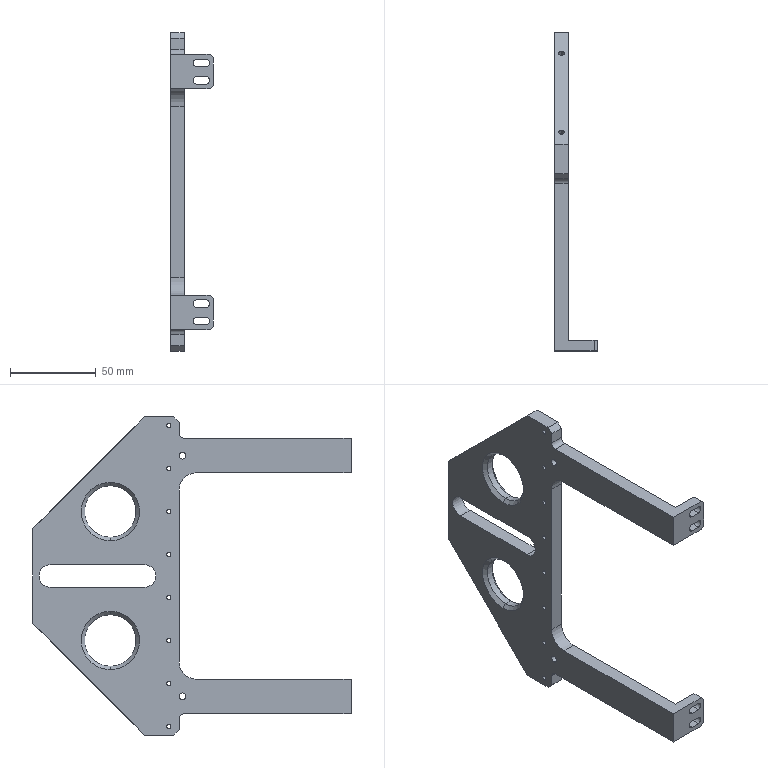Part | SolidWorks | features HoleWzd 4, ICE 4, Chamfer 3, Fillet 2, Extrusion 1, MirrorPattern 1 | 1 solid | 106 faces | box 25 x 185 x 185 mm | volume 107483 mm3 | cylinder 50 | plane 36 | cone 20 | commonest cylinder face diameters 2.5 x16 3.3 x12 4.5 x8 4 x4 30 x4 6 x2